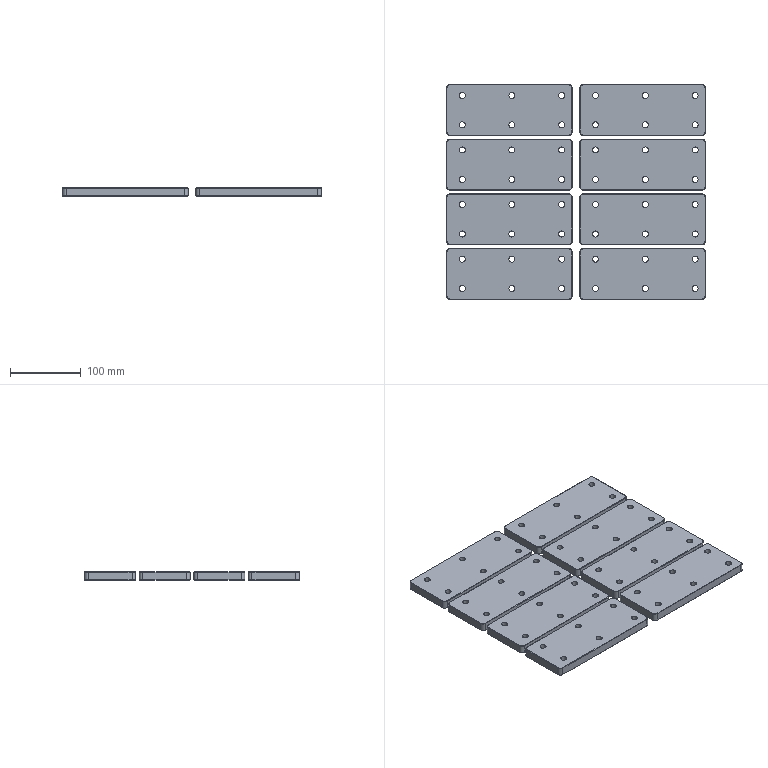Part | 8 solids | 304 faces | box 365 x 303 x 12 mm | volume 1187702 mm3 | cylinder 128 | plane 112 | cone 64 | commonest cylinder face diameters 8.5 x96 10 x32